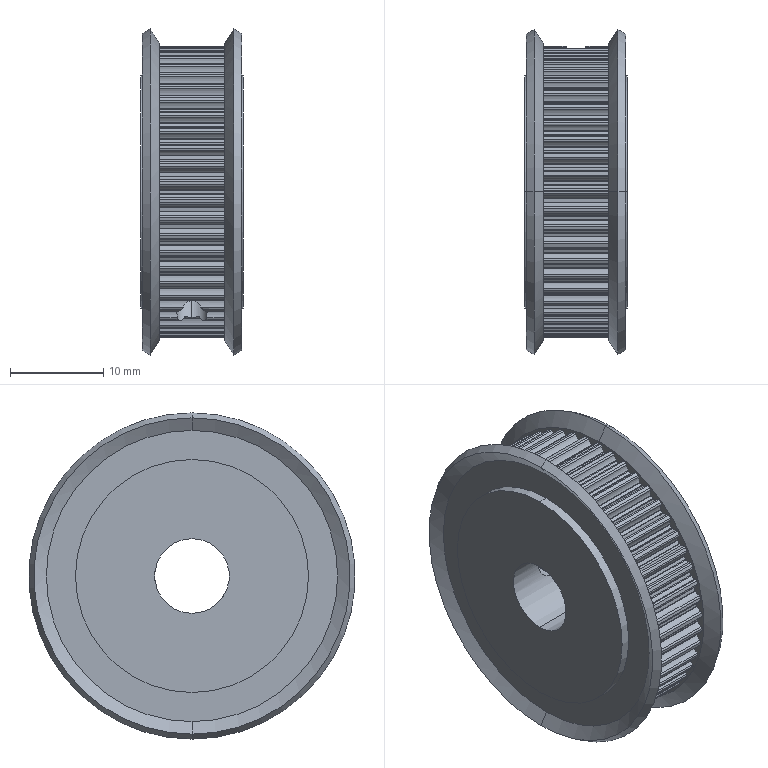Part | SolidWorks | features BaseBody 3, CirPattern 1, HoleWzd 1 | 1 solid | 499 faces | box 11 x 35 x 35 mm | volume 7284 mm3 | cylinder 481 | cone 12 | plane 6 | commonest cylinder face diameters 0.38 x131 0.2 x117 2.65 x115 31.32 x55 29.8 x52 3.3 x4